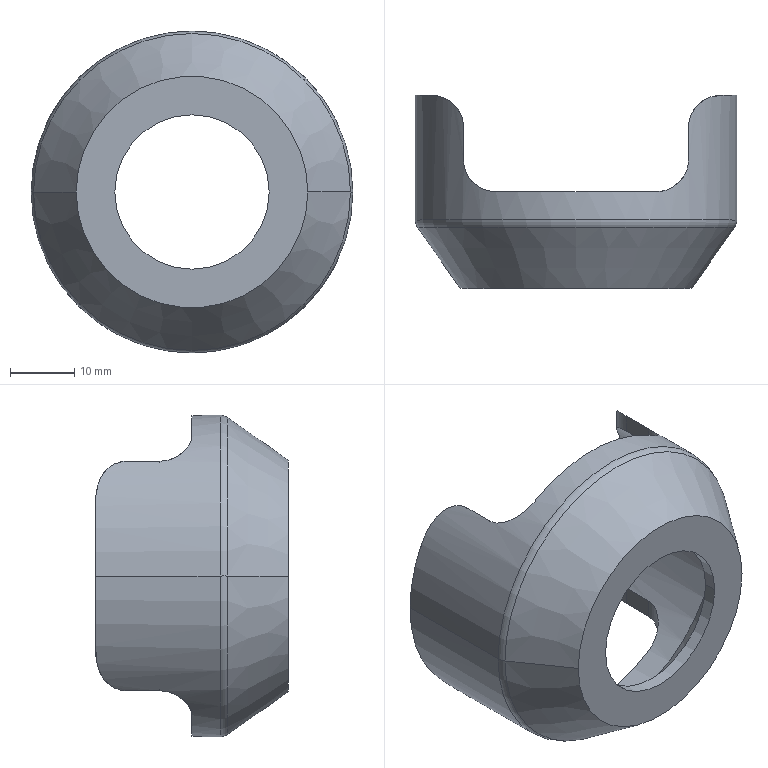Part | STEP file | Schneider emergency stop button guard ZB2BZ1605C | 1 solid | 30 faces | box 50 x 30 x 50 mm | volume 7549 mm3 | cylinder 14 | plane 10 | cone 4 | torus 2 | commonest cylinder face diameters 10 x8 24 x2 46 x2 50 x2